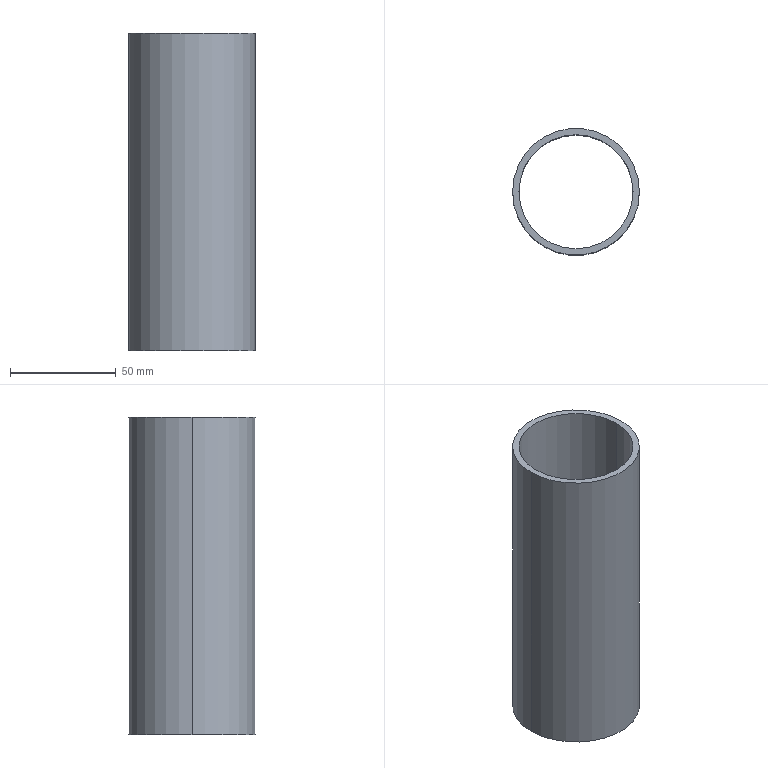Part | SolidWorks | features Extrusion 1 | 1 solid | 6 faces | box 60 x 60 x 150 mm | volume 80582 mm3 | cylinder 4 | plane 2 | commonest cylinder face diameters 54 x2 60 x2
STEP:
#1=CARTESIAN_POINT('',(-27.,0.,150.));
#2=VERTEX_POINT('',#1);
#3=CARTESIAN_POINT('',(27.,0.,150.));
#4=VERTEX_POINT('',#3);
#5=CARTESIAN_POINT('',(0.,0.,150.));
#6=DIRECTION('',(0.,0.,1.));
#7=DIRECTION('',(1.,0.,0.));
#8=AXIS2_PLACEMENT_3D('',#5,#6,#7);
#9=CIRCLE('',#8,27.);
#10=EDGE_CURVE('',#2,#4,#9,.T.);
#11=ORIENTED_EDGE('',*,*,#10,.T.);
#12=CARTESIAN_POINT('',(27.,0.,0.));
#13=VERTEX_POINT('',#12);
#14=CARTESIAN_POINT('',(27.,0.,150.));
#15=DIRECTION('',(0.,0.,-1.));
#16=VECTOR('',#15,1000.);
#17=LINE('',#14,#16);
#18=EDGE_CURVE('',#4,#13,#17,.T.);
#19=ORIENTED_EDGE('',*,*,#18,.T.);
#20=CARTESIAN_POINT('',(-27.,0.,0.));
#21=VERTEX_POINT('',#20);
#22=CARTESIAN_POINT('',(0.,0.,0.));
#23=DIRECTION('',(0.,0.,1.));
#24=DIRECTION('',(1.,0.,0.));
#25=AXIS2_PLACEMENT_3D('',#22,#23,#24);
#26=CIRCLE('',#25,27.);
#27=EDGE_CURVE('',#21,#13,#26,.T.);
#28=ORIENTED_EDGE('',*,*,#27,.F.);
#29=CARTESIAN_POINT('',(-27.,0.,150.));
#30=DIRECTION('',(0.,0.,-1.));
#31=VECTOR('',#30,1000.);
#32=LINE('',#29,#31);
#33=EDGE_CURVE('',#2,#21,#32,.T.);
#34=ORIENTED_EDGE('',*,*,#33,.F.);
#35=EDGE_LOOP('',(#11,#19,#28,#34));
#36=FACE_OUTER_BOUND('',#35,.T.);
#37=CARTESIAN_POINT('',(0.,0.,150.));
#38=DIRECTION('',(0.,0.,-1.));
#39=DIRECTION('',(-1.,0.,0.));
#40=AXIS2_PLACEMENT_3D('',#37,#38,#39);
#41=CYLINDRICAL_SURFACE('',#40,27.);
#42=ADVANCED_FACE('',(#36),#41,.F.);
#43=CARTESIAN_POINT('',(30.,0.,150.));
#44=VERTEX_POINT('',#43);
#45=CARTESIAN_POINT('',(-30.,0.,150.));
#46=VERTEX_POINT('',#45);
#47=CARTESIAN_POINT('',(0.,0.,150.));
#48=DIRECTION('',(0.,0.,1.));
#49=DIRECTION('',(1.,0.,0.));
#50=AXIS2_PLACEMENT_3D('',#47,#48,#49);
#51=CIRCLE('',#50,30.);
#52=EDGE_CURVE('',#44,#46,#51,.T.);
#53=ORIENTED_EDGE('',*,*,#52,.F.);
#54=CARTESIAN_POINT('',(30.,0.,0.));
#55=VERTEX_POINT('',#54);
#56=CARTESIAN_POINT('',(30.,0.,150.));
#57=DIRECTION('',(0.,0.,-1.));
#58=VECTOR('',#57,1000.);
#59=LINE('',#56,#58);
#60=EDGE_CURVE('',#44,#55,#59,.T.);
#61=ORIENTED_EDGE('',*,*,#60,.T.);
#62=CARTESIAN_POINT('',(-30.,0.,0.));
#63=VERTEX_POINT('',#62);
#64=CARTESIAN_POINT('',(0.,0.,0.));
#65=DIRECTION('',(0.,0.,1.));
#66=DIRECTION('',(1.,0.,0.));
#67=AXIS2_PLACEMENT_3D('',#64,#65,#66);
#68=CIRCLE('',#67,30.);
#69=EDGE_CURVE('',#55,#63,#68,.T.);
#70=ORIENTED_EDGE('',*,*,#69,.T.);
#71=CARTESIAN_POINT('',(-30.,0.,150.));
#72=DIRECTION('',(0.,0.,-1.));
#73=VECTOR('',#72,1000.);
#74=LINE('',#71,#73);
#75=EDGE_CURVE('',#46,#63,#74,.T.);
#76=ORIENTED_EDGE('',*,*,#75,.F.);
#77=EDGE_LOOP('',(#53,#61,#70,#76));
#78=FACE_OUTER_BOUND('',#77,.T.);
#79=CARTESIAN_POINT('',(0.,0.,150.));
#80=DIRECTION('',(0.,0.,-1.));
#81=DIRECTION('',(-1.,0.,0.));
#82=AXIS2_PLACEMENT_3D('',#79,#80,#81);
#83=CYLINDRICAL_SURFACE('',#82,30.);
#84=ADVANCED_FACE('',(#78),#83,.T.);
#85=CARTESIAN_POINT('',(0.,0.,150.));
#86=DIRECTION('',(0.,0.,1.));
#87=DIRECTION('',(1.,0.,0.));
#88=AXIS2_PLACEMENT_3D('',#85,#86,#87);
#89=CIRCLE('',#88,30.);
#90=EDGE_CURVE('',#46,#44,#89,.T.);
#91=ORIENTED_EDGE('',*,*,#90,.T.);
#92=ORIENTED_EDGE('',*,*,#52,.T.);
#93=EDGE_LOOP('',(#91,#92));
#94=FACE_OUTER_BOUND('',#93,.T.);
#95=ORIENTED_EDGE('',*,*,#10,.F.);
#96=CARTESIAN_POINT('',(0.,0.,150.));
#97=DIRECTION('',(0.,0.,1.));
#98=DIRECTION('',(1.,0.,0.));
#99=AXIS2_PLACEMENT_3D('',#96,#97,#98);
#100=CIRCLE('',#99,27.);
#101=EDGE_CURVE('',#4,#2,#100,.T.);
#102=ORIENTED_EDGE('',*,*,#101,.F.);
#103=EDGE_LOOP('',(#95,#102));
#104=FACE_BOUND('',#103,.T.);
#105=CARTESIAN_POINT('',(0.,0.,150.));
#106=DIRECTION('',(0.,0.,1.));
#107=DIRECTION('',(1.,0.,0.));
#108=AXIS2_PLACEMENT_3D('',#105,#106,#107);
#109=PLANE('',#108);
#110=ADVANCED_FACE('',(#94,#104),#109,.T.);
#111=CARTESIAN_POINT('',(0.,0.,0.));
#112=DIRECTION('',(0.,0.,1.));
#113=DIRECTION('',(1.,0.,0.));
#114=AXIS2_PLACEMENT_3D('',#111,#112,#113);
#115=CIRCLE('',#114,30.);
#116=EDGE_CURVE('',#63,#55,#115,.T.);
#117=ORIENTED_EDGE('',*,*,#116,.F.);
#118=ORIENTED_EDGE('',*,*,#69,.F.);
#119=EDGE_LOOP('',(#117,#118));
#120=FACE_OUTER_BOUND('',#119,.T.);
#121=ORIENTED_EDGE('',*,*,#27,.T.);
#122=CARTESIAN_POINT('',(0.,0.,0.));
#123=DIRECTION('',(0.,0.,1.));
#124=DIRECTION('',(1.,0.,0.));
#125=AXIS2_PLACEMENT_3D('',#122,#123,#124);
#126=CIRCLE('',#125,27.);
#127=EDGE_CURVE('',#13,#21,#126,.T.);
#128=ORIENTED_EDGE('',*,*,#127,.T.);
#129=EDGE_LOOP('',(#121,#128));
#130=FACE_BOUND('',#129,.T.);
#131=CARTESIAN_POINT('',(0.,0.,0.));
#132=DIRECTION('',(0.,0.,1.));
#133=DIRECTION('',(1.,0.,0.));
#134=AXIS2_PLACEMENT_3D('',#131,#132,#133);
#135=PLANE('',#134);
#136=ADVANCED_FACE('',(#120,#130),#135,.F.);
#137=ORIENTED_EDGE('',*,*,#60,.F.);
#138=ORIENTED_EDGE('',*,*,#90,.F.);
#139=ORIENTED_EDGE('',*,*,#75,.T.);
#140=ORIENTED_EDGE('',*,*,#116,.T.);
#141=EDGE_LOOP('',(#137,#138,#139,#140));
#142=FACE_OUTER_BOUND('',#141,.T.);
#143=CARTESIAN_POINT('',(0.,0.,150.));
#144=DIRECTION('',(0.,0.,-1.));
#145=DIRECTION('',(-1.,0.,0.));
#146=AXIS2_PLACEMENT_3D('',#143,#144,#145);
#147=CYLINDRICAL_SURFACE('',#146,30.);
#148=ADVANCED_FACE('',(#142),#147,.T.);
#149=ORIENTED_EDGE('',*,*,#18,.F.);
#150=ORIENTED_EDGE('',*,*,#101,.T.);
#151=ORIENTED_EDGE('',*,*,#33,.T.);
#152=ORIENTED_EDGE('',*,*,#127,.F.);
#153=EDGE_LOOP('',(#149,#150,#151,#152));
#154=FACE_OUTER_BOUND('',#153,.T.);
#155=CARTESIAN_POINT('',(0.,0.,150.));
#156=DIRECTION('',(0.,0.,-1.));
#157=DIRECTION('',(-1.,0.,0.));
#158=AXIS2_PLACEMENT_3D('',#155,#156,#157);
#159=CYLINDRICAL_SURFACE('',#158,27.);
#160=ADVANCED_FACE('',(#154),#159,.F.);
#161=CLOSED_SHELL('',(#42,#84,#110,#136,#148,#160));
#162=MANIFOLD_SOLID_BREP('',#161);
#163=CARTESIAN_POINT('',(0.,0.,0.));
#164=DIRECTION('',(0.,0.,1.));
#165=DIRECTION('',(1.,0.,0.));
#166=AXIS2_PLACEMENT_3D('',#163,#164,#165);
#167=(LENGTH_UNIT()NAMED_UNIT(*)SI_UNIT(.MILLI.,.METRE.));
#168=UNCERTAINTY_MEASURE_WITH_UNIT(LENGTH_MEASURE(0.00001),#167,'','');
#169=(NAMED_UNIT(*)PLANE_ANGLE_UNIT()SI_UNIT($,.RADIAN.));
#170=(NAMED_UNIT(*)SI_UNIT($,.STERADIAN.)SOLID_ANGLE_UNIT());
#171=(GEOMETRIC_REPRESENTATION_CONTEXT(3)GLOBAL_UNCERTAINTY_ASSIGNED_CONTEXT((#168))GLOBAL_UNIT_ASSIGNED_CONTEXT((#167,#169,#170))REPRESENTATION_CONTEXT('',''));
#172=ADVANCED_BREP_SHAPE_REPRESENTATION('',(#162,#166),#171);